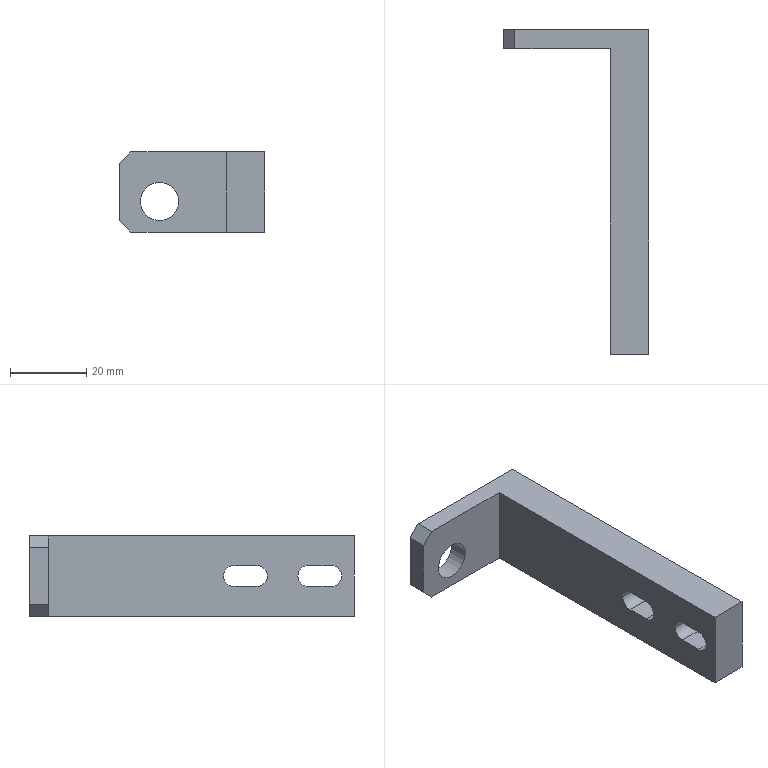Part | STEP file | turning cylinder seat | 1 solid | 30 faces | box 38 x 85 x 21 mm | volume 18885 mm3 | plane 14 | cylinder 12 | cone 4 | commonest cylinder face diameters 5.5 x6 4.5 x4 10 x2